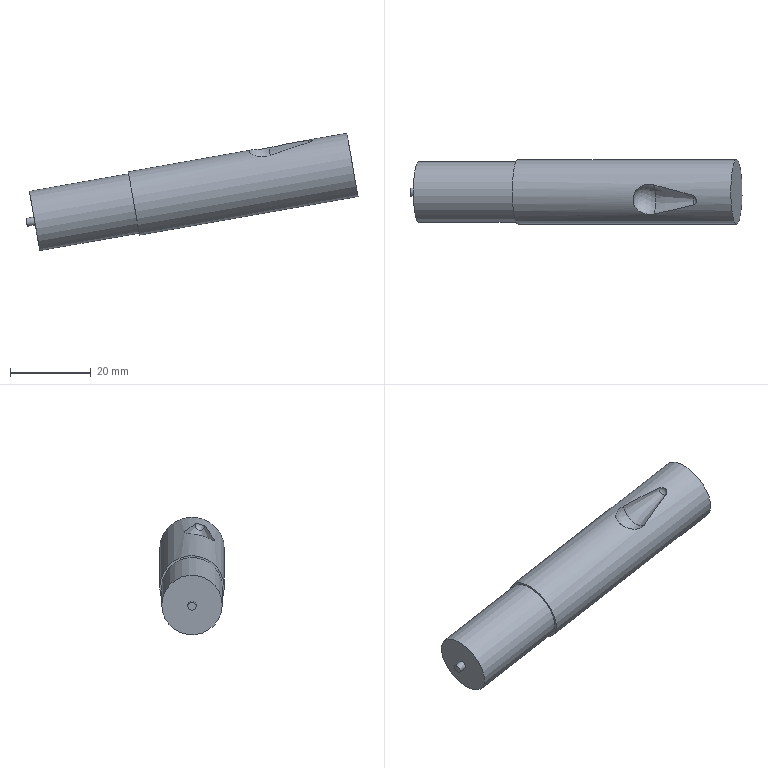Part | NX | features solid 2 | 1 solid | 10 faces | box 82.317 x 16 x 29.156 mm | volume 15294 mm3 | plane 4 | cylinder 3 | sphere 2 | cone 1 | commonest cylinder face diameters 2 x1 15 x1 16 x1
STEP:
#1=CARTESIAN_POINT('',(-555.934,-54.824,25.415));
#2=VERTEX_POINT('',#1);
#3=CARTESIAN_POINT('',(-556.271,-47.58,27.326));
#4=DIRECTION('',(-0.9848,0.,-0.1736));
#5=DIRECTION('',(0.04494,-0.9659,-0.2549));
#6=AXIS2_PLACEMENT_3D('',#3,#4,#5);
#7=CIRCLE('',#6,7.5);
#8=EDGE_CURVE('',#2,#2,#7,.T.);
#9=ORIENTED_EDGE('',*,*,#8,.T.);
#10=EDGE_LOOP('',(#9));
#11=FACE_BOUND('',#10,.T.);
#12=CARTESIAN_POINT('',(-556.098,-47.58,26.341));
#13=VERTEX_POINT('',#12);
#14=CARTESIAN_POINT('',(-556.271,-47.58,27.326));
#15=DIRECTION('',(-0.9848,0.,-0.1736));
#16=DIRECTION('',(0.1736,0.,-0.9848));
#17=AXIS2_PLACEMENT_3D('',#14,#15,#16);
#18=CIRCLE('',#17,1.);
#19=EDGE_CURVE('',#13,#13,#18,.F.);
#20=ORIENTED_EDGE('',*,*,#19,.T.);
#21=EDGE_LOOP('',(#20));
#22=FACE_BOUND('',#21,.T.);
#23=CARTESIAN_POINT('',(-556.271,-47.58,27.326));
#24=DIRECTION('',(0.9848,0.,0.1736));
#25=DIRECTION('',(0.04494,-0.9659,-0.2549));
#26=AXIS2_PLACEMENT_3D('',#23,#24,#25);
#27=PLANE('',#26);
#28=ADVANCED_FACE('',(#11,#22),#27,.F.);
#29=CARTESIAN_POINT('',(-497.87,-53.037,43.563));
#30=VERTEX_POINT('',#29);
#31=CARTESIAN_POINT('',(-488.273,-50.866,46.722));
#32=VERTEX_POINT('',#31);
#33=CARTESIAN_POINT('',(-497.87,-53.037,43.563));
#34=CARTESIAN_POINT('',(-494.696,-52.389,44.737));
#35=CARTESIAN_POINT('',(-491.497,-51.654,45.793));
#36=CARTESIAN_POINT('',(-488.273,-50.866,46.722));
#37=B_SPLINE_CURVE_WITH_KNOTS('',3,(#33,#34,#35,#36),.UNSPECIFIED.,.F.,.F.,(4,4),(0.000000207,0.01034),.UNSPECIFIED.);
#38=EDGE_CURVE('',#30,#32,#37,.T.);
#39=ORIENTED_EDGE('',*,*,#38,.F.);
#40=CARTESIAN_POINT('',(-498.208,-45.778,45.479));
#41=VERTEX_POINT('',#40);
#42=CARTESIAN_POINT('',(-498.208,-45.778,45.479));
#43=CARTESIAN_POINT('',(-499.367,-45.469,45.202));
#44=CARTESIAN_POINT('',(-501.321,-45.888,45.025));
#45=CARTESIAN_POINT('',(-502.897,-47.848,44.919));
#46=CARTESIAN_POINT('',(-503.273,-49.663,44.592));
#47=CARTESIAN_POINT('',(-502.734,-51.375,43.989));
#48=CARTESIAN_POINT('',(-500.996,-52.985,43.153));
#49=CARTESIAN_POINT('',(-499.005,-53.269,43.144));
#50=CARTESIAN_POINT('',(-497.87,-53.037,43.563));
#51=B_SPLINE_CURVE_WITH_KNOTS('',3,(#42,#43,#44,#45,#46,#47,#48,#49,#50),.UNSPECIFIED.,.F.,.F.,(4,1,1,1,1,1,4),(0.000000204,0.003641,0.005462,0.007282,0.009103,0.01092,0.01456),.UNSPECIFIED.);
#52=EDGE_CURVE('',#41,#30,#51,.T.);
#53=ORIENTED_EDGE('',*,*,#52,.F.);
#54=CARTESIAN_POINT('',(-488.389,-48.38,47.378));
#55=VERTEX_POINT('',#54);
#56=CARTESIAN_POINT('',(-488.389,-48.38,47.378));
#57=CARTESIAN_POINT('',(-491.69,-47.52,46.884));
#58=CARTESIAN_POINT('',(-494.963,-46.641,46.254));
#59=CARTESIAN_POINT('',(-498.208,-45.778,45.479));
#60=B_SPLINE_CURVE_WITH_KNOTS('',3,(#56,#57,#58,#59),.UNSPECIFIED.,.F.,.F.,(4,4),(0.000000207,0.01034),.UNSPECIFIED.);
#61=EDGE_CURVE('',#55,#41,#60,.T.);
#62=ORIENTED_EDGE('',*,*,#61,.F.);
#63=CARTESIAN_POINT('',(-488.273,-50.866,46.722));
#64=CARTESIAN_POINT('',(-487.72,-50.731,46.882));
#65=CARTESIAN_POINT('',(-486.956,-49.673,47.473));
#66=CARTESIAN_POINT('',(-487.822,-48.528,47.463));
#67=CARTESIAN_POINT('',(-488.389,-48.38,47.378));
#68=B_SPLINE_CURVE_WITH_KNOTS('',3,(#63,#64,#65,#66,#67),.UNSPECIFIED.,.F.,.F.,(4,1,4),(0.000000204,0.00175,0.003499),.UNSPECIFIED.);
#69=EDGE_CURVE('',#32,#55,#68,.T.);
#70=ORIENTED_EDGE('',*,*,#69,.F.);
#71=EDGE_LOOP('',(#39,#53,#62,#70));
#72=FACE_BOUND('',#71,.T.);
#73=CARTESIAN_POINT('',(-477.127,-55.307,39.179));
#74=VERTEX_POINT('',#73);
#75=CARTESIAN_POINT('',(-477.487,-47.58,41.218));
#76=DIRECTION('',(-0.9848,0.,-0.1736));
#77=DIRECTION('',(0.04494,-0.9659,-0.2549));
#78=AXIS2_PLACEMENT_3D('',#75,#76,#77);
#79=CIRCLE('',#78,8.);
#80=EDGE_CURVE('',#74,#74,#79,.T.);
#81=ORIENTED_EDGE('',*,*,#80,.T.);
#82=EDGE_LOOP('',(#81));
#83=FACE_BOUND('',#82,.T.);
#84=CARTESIAN_POINT('',(-531.292,-55.307,29.628));
#85=VERTEX_POINT('',#84);
#86=CARTESIAN_POINT('',(-531.651,-47.58,31.667));
#87=DIRECTION('',(-0.9848,0.,-0.1736));
#88=DIRECTION('',(0.04494,-0.9659,-0.2549));
#89=AXIS2_PLACEMENT_3D('',#86,#87,#88);
#90=CIRCLE('',#89,8.);
#91=EDGE_CURVE('',#85,#85,#90,.T.);
#92=ORIENTED_EDGE('',*,*,#91,.F.);
#93=EDGE_LOOP('',(#92));
#94=FACE_BOUND('',#93,.T.);
#95=CARTESIAN_POINT('',(-477.487,-47.58,41.218));
#96=DIRECTION('',(-0.9848,0.,-0.1736));
#97=DIRECTION('',(-0.04494,0.9659,0.2549));
#98=AXIS2_PLACEMENT_3D('',#95,#96,#97);
#99=CYLINDRICAL_SURFACE('',#98,8.);
#100=ADVANCED_FACE('',(#72,#83,#94),#99,.T.);
#101=ORIENTED_EDGE('',*,*,#80,.F.);
#102=EDGE_LOOP('',(#101));
#103=FACE_BOUND('',#102,.T.);
#104=CARTESIAN_POINT('',(-477.487,-47.58,41.218));
#105=DIRECTION('',(0.9848,0.,0.1736));
#106=DIRECTION('',(0.04494,-0.9659,-0.2549));
#107=AXIS2_PLACEMENT_3D('',#104,#105,#106);
#108=PLANE('',#107);
#109=ADVANCED_FACE('',(#103),#108,.T.);
#110=CARTESIAN_POINT('',(-531.314,-54.824,29.756));
#111=VERTEX_POINT('',#110);
#112=CARTESIAN_POINT('',(-531.651,-47.58,31.667));
#113=DIRECTION('',(-0.9848,0.,-0.1736));
#114=DIRECTION('',(0.04494,-0.9659,-0.2549));
#115=AXIS2_PLACEMENT_3D('',#112,#113,#114);
#116=CIRCLE('',#115,7.5);
#117=EDGE_CURVE('',#111,#111,#116,.T.);
#118=ORIENTED_EDGE('',*,*,#117,.F.);
#119=EDGE_LOOP('',(#118));
#120=FACE_BOUND('',#119,.T.);
#121=ORIENTED_EDGE('',*,*,#91,.T.);
#122=EDGE_LOOP('',(#121));
#123=FACE_BOUND('',#122,.T.);
#124=CARTESIAN_POINT('',(-531.651,-47.58,31.667));
#125=DIRECTION('',(0.9848,0.,0.1736));
#126=DIRECTION('',(0.04494,-0.9659,-0.2549));
#127=AXIS2_PLACEMENT_3D('',#124,#125,#126);
#128=PLANE('',#127);
#129=ADVANCED_FACE('',(#120,#123),#128,.F.);
#130=ORIENTED_EDGE('',*,*,#8,.F.);
#131=EDGE_LOOP('',(#130));
#132=FACE_BOUND('',#131,.T.);
#133=ORIENTED_EDGE('',*,*,#117,.T.);
#134=EDGE_LOOP('',(#133));
#135=FACE_BOUND('',#134,.T.);
#136=CARTESIAN_POINT('',(-556.271,-47.58,27.326));
#137=DIRECTION('',(0.9848,0.,0.1736));
#138=DIRECTION('',(0.04494,-0.9659,-0.2549));
#139=AXIS2_PLACEMENT_3D('',#136,#137,#138);
#140=CYLINDRICAL_SURFACE('',#139,7.5);
#141=ADVANCED_FACE('',(#132,#135),#140,.T.);
#142=CARTESIAN_POINT('',(-498.197,-49.65,45.413));
#143=DIRECTION('',(0.9848,0.,0.1736));
#144=DIRECTION('',(-0.04494,0.9659,0.2549));
#145=AXIS2_PLACEMENT_3D('',#142,#143,#144);
#146=CIRCLE('',#145,3.873);
#147=EDGE_CURVE('',#30,#41,#146,.T.);
#148=ORIENTED_EDGE('',*,*,#147,.T.);
#149=ORIENTED_EDGE('',*,*,#52,.T.);
#150=EDGE_LOOP('',(#148,#149));
#151=FACE_BOUND('',#150,.T.);
#152=CARTESIAN_POINT('',(-499.181,-49.65,45.239));
#153=DIRECTION('',(-0.9848,0.,-0.1736));
#154=DIRECTION('',(-0.04494,0.9659,0.2549));
#155=AXIS2_PLACEMENT_3D('',#152,#153,#154);
#156=SPHERICAL_SURFACE('',#155,4.);
#157=ADVANCED_FACE('',(#151),#156,.F.);
#158=CARTESIAN_POINT('',(-488.348,-49.65,47.149));
#159=DIRECTION('',(0.9848,0.,0.1736));
#160=DIRECTION('',(-0.04494,0.9659,0.2549));
#161=AXIS2_PLACEMENT_3D('',#158,#159,#160);
#162=CIRCLE('',#161,1.291);
#163=EDGE_CURVE('',#32,#55,#162,.T.);
#164=ORIENTED_EDGE('',*,*,#163,.T.);
#165=ORIENTED_EDGE('',*,*,#61,.T.);
#166=ORIENTED_EDGE('',*,*,#147,.F.);
#167=ORIENTED_EDGE('',*,*,#38,.T.);
#168=EDGE_LOOP('',(#164,#165,#166,#167));
#169=FACE_BOUND('',#168,.T.);
#170=CARTESIAN_POINT('',(-498.197,-49.65,45.413));
#171=DIRECTION('',(-0.9848,0.,-0.1736));
#172=DIRECTION('',(-0.04494,0.9659,0.2549));
#173=AXIS2_PLACEMENT_3D('',#170,#171,#172);
#174=CONICAL_SURFACE('',#173,3.873,0.2527);
#175=ADVANCED_FACE('',(#169),#174,.F.);
#176=ORIENTED_EDGE('',*,*,#163,.F.);
#177=ORIENTED_EDGE('',*,*,#69,.T.);
#178=EDGE_LOOP('',(#176,#177));
#179=FACE_BOUND('',#178,.T.);
#180=CARTESIAN_POINT('',(-488.677,-49.65,47.092));
#181=DIRECTION('',(-0.9848,0.,-0.1736));
#182=DIRECTION('',(0.04494,-0.9659,-0.2549));
#183=AXIS2_PLACEMENT_3D('',#180,#181,#182);
#184=SPHERICAL_SURFACE('',#183,1.333);
#185=ADVANCED_FACE('',(#179),#184,.F.);
#186=ORIENTED_EDGE('',*,*,#19,.F.);
#187=EDGE_LOOP('',(#186));
#188=FACE_BOUND('',#187,.T.);
#189=CARTESIAN_POINT('',(-558.067,-47.58,25.994));
#190=VERTEX_POINT('',#189);
#191=CARTESIAN_POINT('',(-558.241,-47.58,26.979));
#192=DIRECTION('',(-0.9848,0.,-0.1736));
#193=DIRECTION('',(0.1736,0.,-0.9848));
#194=AXIS2_PLACEMENT_3D('',#191,#192,#193);
#195=CIRCLE('',#194,1.);
#196=EDGE_CURVE('',#190,#190,#195,.T.);
#197=ORIENTED_EDGE('',*,*,#196,.F.);
#198=EDGE_LOOP('',(#197));
#199=FACE_BOUND('',#198,.T.);
#200=CARTESIAN_POINT('',(-556.271,-47.58,27.326));
#201=DIRECTION('',(-0.9848,0.,-0.1736));
#202=DIRECTION('',(-0.1736,0.,0.9848));
#203=AXIS2_PLACEMENT_3D('',#200,#201,#202);
#204=CYLINDRICAL_SURFACE('',#203,1.);
#205=ADVANCED_FACE('',(#188,#199),#204,.T.);
#206=ORIENTED_EDGE('',*,*,#196,.T.);
#207=EDGE_LOOP('',(#206));
#208=FACE_BOUND('',#207,.T.);
#209=CARTESIAN_POINT('',(-558.241,-47.58,26.979));
#210=DIRECTION('',(0.9848,0.,0.1736));
#211=DIRECTION('',(0.04494,-0.9659,-0.2549));
#212=AXIS2_PLACEMENT_3D('',#209,#210,#211);
#213=PLANE('',#212);
#214=ADVANCED_FACE('',(#208),#213,.F.);
#215=CLOSED_SHELL('',(#28,#100,#109,#129,#141,#157,#175,#185,#205,#214));
#216=MANIFOLD_SOLID_BREP('',#215);
#217=(LENGTH_UNIT()NAMED_UNIT(*)SI_UNIT(.MILLI.,.METRE.));
#218=UNCERTAINTY_MEASURE_WITH_UNIT(LENGTH_MEASURE(0.0508),#217,'','');
#219=(NAMED_UNIT(*)PLANE_ANGLE_UNIT()SI_UNIT($,.RADIAN.));
#220=(NAMED_UNIT(*)SI_UNIT($,.STERADIAN.)SOLID_ANGLE_UNIT());
#221=(GEOMETRIC_REPRESENTATION_CONTEXT(3)GLOBAL_UNCERTAINTY_ASSIGNED_CONTEXT((#218))GLOBAL_UNIT_ASSIGNED_CONTEXT((#217,#219,#220))REPRESENTATION_CONTEXT('',''));
#222=ADVANCED_BREP_SHAPE_REPRESENTATION('',(#216),#221);